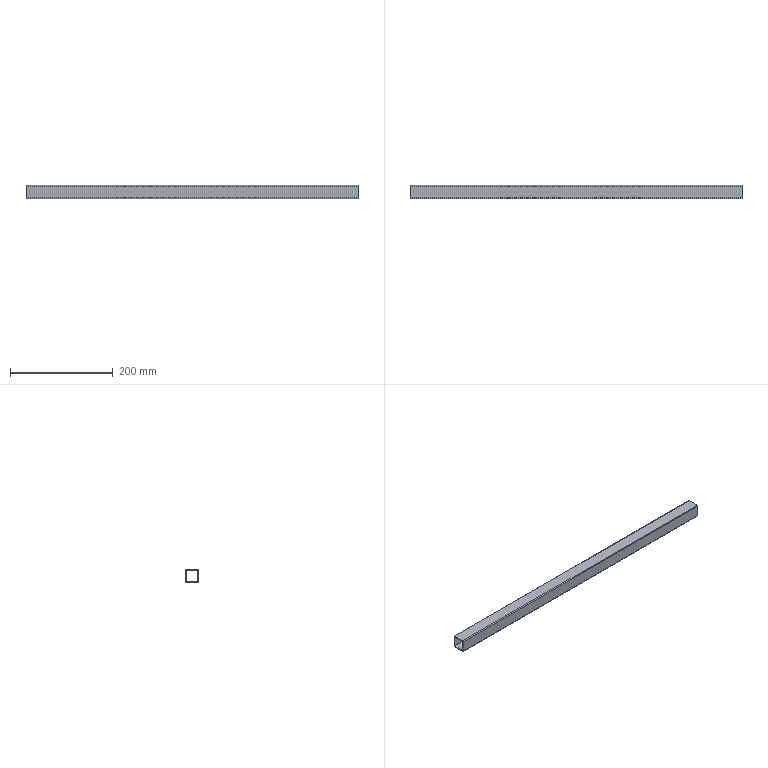Part | NX | features BREP 1 | 1 solid | 14 faces | box 647.7 x 25.4 x 25.4 mm | volume 113135 mm3 | plane 10 | cylinder 4 | commonest cylinder face diameters 3.175 x4
STEP:
#1=CARTESIAN_POINT('',(-323.85,12.7,-11.113));
#2=VERTEX_POINT('',#1);
#3=CARTESIAN_POINT('',(-323.85,12.7,11.113));
#4=VERTEX_POINT('',#3);
#5=CARTESIAN_POINT('',(-323.85,12.7,-11.113));
#6=DIRECTION('',(0.,0.,1.));
#7=VECTOR('',#6,1000.);
#8=LINE('',#5,#7);
#9=EDGE_CURVE('',#2,#4,#8,.T.);
#10=ORIENTED_EDGE('',*,*,#9,.F.);
#11=CARTESIAN_POINT('',(-323.85,11.113,-12.7));
#12=VERTEX_POINT('',#11);
#13=CARTESIAN_POINT('',(-323.85,11.113,-11.113));
#14=DIRECTION('',(-1.,0.,0.));
#15=DIRECTION('',(0.,1.,0.));
#16=AXIS2_PLACEMENT_3D('',#13,#14,#15);
#17=CIRCLE('',#16,1.587);
#18=EDGE_CURVE('',#2,#12,#17,.T.);
#19=ORIENTED_EDGE('',*,*,#18,.T.);
#20=CARTESIAN_POINT('',(-323.85,-11.113,-12.7));
#21=VERTEX_POINT('',#20);
#22=CARTESIAN_POINT('',(-323.85,-11.113,-12.7));
#23=DIRECTION('',(0.,1.,0.));
#24=VECTOR('',#23,1000.);
#25=LINE('',#22,#24);
#26=EDGE_CURVE('',#21,#12,#25,.T.);
#27=ORIENTED_EDGE('',*,*,#26,.F.);
#28=CARTESIAN_POINT('',(-323.85,-12.7,-11.113));
#29=VERTEX_POINT('',#28);
#30=CARTESIAN_POINT('',(-323.85,-11.113,-11.113));
#31=DIRECTION('',(-1.,0.,0.));
#32=DIRECTION('',(0.,0.,-1.));
#33=AXIS2_PLACEMENT_3D('',#30,#31,#32);
#34=CIRCLE('',#33,1.587);
#35=EDGE_CURVE('',#21,#29,#34,.T.);
#36=ORIENTED_EDGE('',*,*,#35,.T.);
#37=CARTESIAN_POINT('',(-323.85,-12.7,11.113));
#38=VERTEX_POINT('',#37);
#39=CARTESIAN_POINT('',(-323.85,-12.7,11.113));
#40=DIRECTION('',(0.,0.,-1.));
#41=VECTOR('',#40,1000.);
#42=LINE('',#39,#41);
#43=EDGE_CURVE('',#38,#29,#42,.T.);
#44=ORIENTED_EDGE('',*,*,#43,.F.);
#45=CARTESIAN_POINT('',(-323.85,-11.113,12.7));
#46=VERTEX_POINT('',#45);
#47=CARTESIAN_POINT('',(-323.85,-11.113,11.113));
#48=DIRECTION('',(-1.,0.,0.));
#49=DIRECTION('',(0.,-1.,0.));
#50=AXIS2_PLACEMENT_3D('',#47,#48,#49);
#51=CIRCLE('',#50,1.587);
#52=EDGE_CURVE('',#38,#46,#51,.T.);
#53=ORIENTED_EDGE('',*,*,#52,.T.);
#54=CARTESIAN_POINT('',(-323.85,11.113,12.7));
#55=VERTEX_POINT('',#54);
#56=CARTESIAN_POINT('',(-323.85,11.113,12.7));
#57=DIRECTION('',(0.,-1.,0.));
#58=VECTOR('',#57,1000.);
#59=LINE('',#56,#58);
#60=EDGE_CURVE('',#55,#46,#59,.T.);
#61=ORIENTED_EDGE('',*,*,#60,.F.);
#62=CARTESIAN_POINT('',(-323.85,11.113,11.113));
#63=DIRECTION('',(-1.,0.,0.));
#64=DIRECTION('',(0.,0.,1.));
#65=AXIS2_PLACEMENT_3D('',#62,#63,#64);
#66=CIRCLE('',#65,1.587);
#67=EDGE_CURVE('',#55,#4,#66,.T.);
#68=ORIENTED_EDGE('',*,*,#67,.T.);
#69=EDGE_LOOP('',(#10,#19,#27,#36,#44,#53,#61,#68));
#70=FACE_BOUND('',#69,.T.);
#71=CARTESIAN_POINT('',(-323.85,10.82,10.82));
#72=VERTEX_POINT('',#71);
#73=CARTESIAN_POINT('',(-323.85,10.82,-10.82));
#74=VERTEX_POINT('',#73);
#75=CARTESIAN_POINT('',(-323.85,10.82,10.82));
#76=DIRECTION('',(0.,0.,-1.));
#77=VECTOR('',#76,1000.);
#78=LINE('',#75,#77);
#79=EDGE_CURVE('',#72,#74,#78,.T.);
#80=ORIENTED_EDGE('',*,*,#79,.F.);
#81=CARTESIAN_POINT('',(-323.85,-10.82,10.82));
#82=VERTEX_POINT('',#81);
#83=CARTESIAN_POINT('',(-323.85,-10.82,10.82));
#84=DIRECTION('',(0.,1.,0.));
#85=VECTOR('',#84,1000.);
#86=LINE('',#83,#85);
#87=EDGE_CURVE('',#82,#72,#86,.T.);
#88=ORIENTED_EDGE('',*,*,#87,.F.);
#89=CARTESIAN_POINT('',(-323.85,-10.82,-10.82));
#90=VERTEX_POINT('',#89);
#91=CARTESIAN_POINT('',(-323.85,-10.82,-10.82));
#92=DIRECTION('',(0.,0.,1.));
#93=VECTOR('',#92,1000.);
#94=LINE('',#91,#93);
#95=EDGE_CURVE('',#90,#82,#94,.T.);
#96=ORIENTED_EDGE('',*,*,#95,.F.);
#97=CARTESIAN_POINT('',(-323.85,10.82,-10.82));
#98=DIRECTION('',(0.,-1.,0.));
#99=VECTOR('',#98,1000.);
#100=LINE('',#97,#99);
#101=EDGE_CURVE('',#74,#90,#100,.T.);
#102=ORIENTED_EDGE('',*,*,#101,.F.);
#103=EDGE_LOOP('',(#80,#88,#96,#102));
#104=FACE_BOUND('',#103,.T.);
#105=CARTESIAN_POINT('',(-323.85,0.,0.));
#106=DIRECTION('',(1.,0.,0.));
#107=DIRECTION('',(0.,1.,0.));
#108=AXIS2_PLACEMENT_3D('',#105,#106,#107);
#109=PLANE('',#108);
#110=ADVANCED_FACE('',(#70,#104),#109,.F.);
#111=CARTESIAN_POINT('',(323.85,-10.82,-10.82));
#112=VERTEX_POINT('',#111);
#113=CARTESIAN_POINT('',(-323.85,-10.82,-10.82));
#114=DIRECTION('',(1.,0.,0.));
#115=VECTOR('',#114,1000.);
#116=LINE('',#113,#115);
#117=EDGE_CURVE('',#90,#112,#116,.T.);
#118=ORIENTED_EDGE('',*,*,#117,.T.);
#119=CARTESIAN_POINT('',(323.85,10.82,-10.82));
#120=VERTEX_POINT('',#119);
#121=CARTESIAN_POINT('',(323.85,10.82,-10.82));
#122=DIRECTION('',(0.,-1.,0.));
#123=VECTOR('',#122,1000.);
#124=LINE('',#121,#123);
#125=EDGE_CURVE('',#120,#112,#124,.T.);
#126=ORIENTED_EDGE('',*,*,#125,.F.);
#127=CARTESIAN_POINT('',(-323.85,10.82,-10.82));
#128=DIRECTION('',(1.,0.,0.));
#129=VECTOR('',#128,1000.);
#130=LINE('',#127,#129);
#131=EDGE_CURVE('',#74,#120,#130,.T.);
#132=ORIENTED_EDGE('',*,*,#131,.F.);
#133=ORIENTED_EDGE('',*,*,#101,.T.);
#134=EDGE_LOOP('',(#118,#126,#132,#133));
#135=FACE_BOUND('',#134,.T.);
#136=CARTESIAN_POINT('',(-323.85,10.82,-10.82));
#137=DIRECTION('',(0.,0.,1.));
#138=DIRECTION('',(1.,0.,0.));
#139=AXIS2_PLACEMENT_3D('',#136,#137,#138);
#140=PLANE('',#139);
#141=ADVANCED_FACE('',(#135),#140,.T.);
#142=ORIENTED_EDGE('',*,*,#131,.T.);
#143=CARTESIAN_POINT('',(323.85,10.82,10.82));
#144=VERTEX_POINT('',#143);
#145=CARTESIAN_POINT('',(323.85,10.82,10.82));
#146=DIRECTION('',(0.,0.,-1.));
#147=VECTOR('',#146,1000.);
#148=LINE('',#145,#147);
#149=EDGE_CURVE('',#144,#120,#148,.T.);
#150=ORIENTED_EDGE('',*,*,#149,.F.);
#151=CARTESIAN_POINT('',(-323.85,10.82,10.82));
#152=DIRECTION('',(1.,0.,0.));
#153=VECTOR('',#152,1000.);
#154=LINE('',#151,#153);
#155=EDGE_CURVE('',#72,#144,#154,.T.);
#156=ORIENTED_EDGE('',*,*,#155,.F.);
#157=ORIENTED_EDGE('',*,*,#79,.T.);
#158=EDGE_LOOP('',(#142,#150,#156,#157));
#159=FACE_BOUND('',#158,.T.);
#160=CARTESIAN_POINT('',(-323.85,10.82,10.82));
#161=DIRECTION('',(0.,-1.,0.));
#162=DIRECTION('',(0.,0.,-1.));
#163=AXIS2_PLACEMENT_3D('',#160,#161,#162);
#164=PLANE('',#163);
#165=ADVANCED_FACE('',(#159),#164,.T.);
#166=ORIENTED_EDGE('',*,*,#155,.T.);
#167=CARTESIAN_POINT('',(323.85,-10.82,10.82));
#168=VERTEX_POINT('',#167);
#169=CARTESIAN_POINT('',(323.85,-10.82,10.82));
#170=DIRECTION('',(0.,1.,0.));
#171=VECTOR('',#170,1000.);
#172=LINE('',#169,#171);
#173=EDGE_CURVE('',#168,#144,#172,.T.);
#174=ORIENTED_EDGE('',*,*,#173,.F.);
#175=CARTESIAN_POINT('',(-323.85,-10.82,10.82));
#176=DIRECTION('',(1.,0.,0.));
#177=VECTOR('',#176,1000.);
#178=LINE('',#175,#177);
#179=EDGE_CURVE('',#82,#168,#178,.T.);
#180=ORIENTED_EDGE('',*,*,#179,.F.);
#181=ORIENTED_EDGE('',*,*,#87,.T.);
#182=EDGE_LOOP('',(#166,#174,#180,#181));
#183=FACE_BOUND('',#182,.T.);
#184=CARTESIAN_POINT('',(-323.85,-10.82,10.82));
#185=DIRECTION('',(0.,0.,-1.));
#186=DIRECTION('',(0.,-1.,0.));
#187=AXIS2_PLACEMENT_3D('',#184,#185,#186);
#188=PLANE('',#187);
#189=ADVANCED_FACE('',(#183),#188,.T.);
#190=ORIENTED_EDGE('',*,*,#179,.T.);
#191=CARTESIAN_POINT('',(323.85,-10.82,-10.82));
#192=DIRECTION('',(0.,0.,1.));
#193=VECTOR('',#192,1000.);
#194=LINE('',#191,#193);
#195=EDGE_CURVE('',#112,#168,#194,.T.);
#196=ORIENTED_EDGE('',*,*,#195,.F.);
#197=ORIENTED_EDGE('',*,*,#117,.F.);
#198=ORIENTED_EDGE('',*,*,#95,.T.);
#199=EDGE_LOOP('',(#190,#196,#197,#198));
#200=FACE_BOUND('',#199,.T.);
#201=CARTESIAN_POINT('',(-323.85,-10.82,-10.82));
#202=DIRECTION('',(0.,1.,0.));
#203=DIRECTION('',(1.,0.,0.));
#204=AXIS2_PLACEMENT_3D('',#201,#202,#203);
#205=PLANE('',#204);
#206=ADVANCED_FACE('',(#200),#205,.T.);
#207=CARTESIAN_POINT('',(323.85,11.113,12.7));
#208=VERTEX_POINT('',#207);
#209=CARTESIAN_POINT('',(323.85,-11.113,12.7));
#210=VERTEX_POINT('',#209);
#211=CARTESIAN_POINT('',(323.85,11.113,12.7));
#212=DIRECTION('',(0.,-1.,0.));
#213=VECTOR('',#212,1000.);
#214=LINE('',#211,#213);
#215=EDGE_CURVE('',#208,#210,#214,.T.);
#216=ORIENTED_EDGE('',*,*,#215,.T.);
#217=CARTESIAN_POINT('',(323.85,-12.7,11.113));
#218=VERTEX_POINT('',#217);
#219=CARTESIAN_POINT('',(323.85,-11.113,11.113));
#220=DIRECTION('',(1.,0.,0.));
#221=DIRECTION('',(0.,0.,1.));
#222=AXIS2_PLACEMENT_3D('',#219,#220,#221);
#223=CIRCLE('',#222,1.587);
#224=EDGE_CURVE('',#210,#218,#223,.T.);
#225=ORIENTED_EDGE('',*,*,#224,.T.);
#226=CARTESIAN_POINT('',(323.85,-12.7,-11.113));
#227=VERTEX_POINT('',#226);
#228=CARTESIAN_POINT('',(323.85,-12.7,11.113));
#229=DIRECTION('',(0.,0.,-1.));
#230=VECTOR('',#229,1000.);
#231=LINE('',#228,#230);
#232=EDGE_CURVE('',#218,#227,#231,.T.);
#233=ORIENTED_EDGE('',*,*,#232,.T.);
#234=CARTESIAN_POINT('',(323.85,-11.113,-12.7));
#235=VERTEX_POINT('',#234);
#236=CARTESIAN_POINT('',(323.85,-11.113,-11.113));
#237=DIRECTION('',(1.,0.,0.));
#238=DIRECTION('',(0.,-1.,0.));
#239=AXIS2_PLACEMENT_3D('',#236,#237,#238);
#240=CIRCLE('',#239,1.587);
#241=EDGE_CURVE('',#227,#235,#240,.T.);
#242=ORIENTED_EDGE('',*,*,#241,.T.);
#243=CARTESIAN_POINT('',(323.85,11.113,-12.7));
#244=VERTEX_POINT('',#243);
#245=CARTESIAN_POINT('',(323.85,-11.113,-12.7));
#246=DIRECTION('',(0.,1.,0.));
#247=VECTOR('',#246,1000.);
#248=LINE('',#245,#247);
#249=EDGE_CURVE('',#235,#244,#248,.T.);
#250=ORIENTED_EDGE('',*,*,#249,.T.);
#251=CARTESIAN_POINT('',(323.85,12.7,-11.113));
#252=VERTEX_POINT('',#251);
#253=CARTESIAN_POINT('',(323.85,11.113,-11.113));
#254=DIRECTION('',(1.,0.,0.));
#255=DIRECTION('',(0.,0.,-1.));
#256=AXIS2_PLACEMENT_3D('',#253,#254,#255);
#257=CIRCLE('',#256,1.587);
#258=EDGE_CURVE('',#244,#252,#257,.T.);
#259=ORIENTED_EDGE('',*,*,#258,.T.);
#260=CARTESIAN_POINT('',(323.85,12.7,11.113));
#261=VERTEX_POINT('',#260);
#262=CARTESIAN_POINT('',(323.85,12.7,-11.113));
#263=DIRECTION('',(0.,0.,1.));
#264=VECTOR('',#263,1000.);
#265=LINE('',#262,#264);
#266=EDGE_CURVE('',#252,#261,#265,.T.);
#267=ORIENTED_EDGE('',*,*,#266,.T.);
#268=CARTESIAN_POINT('',(323.85,11.113,11.113));
#269=DIRECTION('',(1.,0.,0.));
#270=DIRECTION('',(0.,1.,0.));
#271=AXIS2_PLACEMENT_3D('',#268,#269,#270);
#272=CIRCLE('',#271,1.587);
#273=EDGE_CURVE('',#261,#208,#272,.T.);
#274=ORIENTED_EDGE('',*,*,#273,.T.);
#275=EDGE_LOOP('',(#216,#225,#233,#242,#250,#259,#267,#274));
#276=FACE_BOUND('',#275,.T.);
#277=ORIENTED_EDGE('',*,*,#195,.T.);
#278=ORIENTED_EDGE('',*,*,#173,.T.);
#279=ORIENTED_EDGE('',*,*,#149,.T.);
#280=ORIENTED_EDGE('',*,*,#125,.T.);
#281=EDGE_LOOP('',(#277,#278,#279,#280));
#282=FACE_BOUND('',#281,.T.);
#283=CARTESIAN_POINT('',(323.85,0.,0.));
#284=DIRECTION('',(1.,0.,0.));
#285=DIRECTION('',(0.,1.,0.));
#286=AXIS2_PLACEMENT_3D('',#283,#284,#285);
#287=PLANE('',#286);
#288=ADVANCED_FACE('',(#276,#282),#287,.T.);
#289=ORIENTED_EDGE('',*,*,#273,.F.);
#290=CARTESIAN_POINT('',(323.85,12.7,11.113));
#291=DIRECTION('',(-1.,0.,0.));
#292=VECTOR('',#291,1000.);
#293=LINE('',#290,#292);
#294=EDGE_CURVE('',#261,#4,#293,.T.);
#295=ORIENTED_EDGE('',*,*,#294,.T.);
#296=ORIENTED_EDGE('',*,*,#67,.F.);
#297=CARTESIAN_POINT('',(323.85,11.113,12.7));
#298=DIRECTION('',(-1.,0.,0.));
#299=VECTOR('',#298,1000.);
#300=LINE('',#297,#299);
#301=EDGE_CURVE('',#208,#55,#300,.T.);
#302=ORIENTED_EDGE('',*,*,#301,.F.);
#303=EDGE_LOOP('',(#289,#295,#296,#302));
#304=FACE_BOUND('',#303,.T.);
#305=CARTESIAN_POINT('',(324.865,11.113,11.113));
#306=DIRECTION('',(-1.,0.,0.));
#307=DIRECTION('',(0.,0.,1.));
#308=AXIS2_PLACEMENT_3D('',#305,#306,#307);
#309=CYLINDRICAL_SURFACE('',#308,1.587);
#310=ADVANCED_FACE('',(#304),#309,.T.);
#311=ORIENTED_EDGE('',*,*,#60,.T.);
#312=CARTESIAN_POINT('',(323.85,-11.113,12.7));
#313=DIRECTION('',(-1.,0.,0.));
#314=VECTOR('',#313,1000.);
#315=LINE('',#312,#314);
#316=EDGE_CURVE('',#210,#46,#315,.T.);
#317=ORIENTED_EDGE('',*,*,#316,.F.);
#318=ORIENTED_EDGE('',*,*,#215,.F.);
#319=ORIENTED_EDGE('',*,*,#301,.T.);
#320=EDGE_LOOP('',(#311,#317,#318,#319));
#321=FACE_BOUND('',#320,.T.);
#322=CARTESIAN_POINT('',(-323.85,12.7,12.7));
#323=DIRECTION('',(0.,0.,1.));
#324=DIRECTION('',(1.,0.,0.));
#325=AXIS2_PLACEMENT_3D('',#322,#323,#324);
#326=PLANE('',#325);
#327=ADVANCED_FACE('',(#321),#326,.T.);
#328=ORIENTED_EDGE('',*,*,#224,.F.);
#329=ORIENTED_EDGE('',*,*,#316,.T.);
#330=ORIENTED_EDGE('',*,*,#52,.F.);
#331=CARTESIAN_POINT('',(323.85,-12.7,11.113));
#332=DIRECTION('',(-1.,0.,0.));
#333=VECTOR('',#332,1000.);
#334=LINE('',#331,#333);
#335=EDGE_CURVE('',#218,#38,#334,.T.);
#336=ORIENTED_EDGE('',*,*,#335,.F.);
#337=EDGE_LOOP('',(#328,#329,#330,#336));
#338=FACE_BOUND('',#337,.T.);
#339=CARTESIAN_POINT('',(324.865,-11.113,11.113));
#340=DIRECTION('',(-1.,0.,0.));
#341=DIRECTION('',(0.,-1.,0.));
#342=AXIS2_PLACEMENT_3D('',#339,#340,#341);
#343=CYLINDRICAL_SURFACE('',#342,1.587);
#344=ADVANCED_FACE('',(#338),#343,.T.);
#345=ORIENTED_EDGE('',*,*,#43,.T.);
#346=CARTESIAN_POINT('',(323.85,-12.7,-11.113));
#347=DIRECTION('',(-1.,0.,0.));
#348=VECTOR('',#347,1000.);
#349=LINE('',#346,#348);
#350=EDGE_CURVE('',#227,#29,#349,.T.);
#351=ORIENTED_EDGE('',*,*,#350,.F.);
#352=ORIENTED_EDGE('',*,*,#232,.F.);
#353=ORIENTED_EDGE('',*,*,#335,.T.);
#354=EDGE_LOOP('',(#345,#351,#352,#353));
#355=FACE_BOUND('',#354,.T.);
#356=CARTESIAN_POINT('',(-323.85,-12.7,12.7));
#357=DIRECTION('',(0.,-1.,0.));
#358=DIRECTION('',(0.,0.,-1.));
#359=AXIS2_PLACEMENT_3D('',#356,#357,#358);
#360=PLANE('',#359);
#361=ADVANCED_FACE('',(#355),#360,.T.);
#362=ORIENTED_EDGE('',*,*,#241,.F.);
#363=ORIENTED_EDGE('',*,*,#350,.T.);
#364=ORIENTED_EDGE('',*,*,#35,.F.);
#365=CARTESIAN_POINT('',(323.85,-11.113,-12.7));
#366=DIRECTION('',(-1.,0.,0.));
#367=VECTOR('',#366,1000.);
#368=LINE('',#365,#367);
#369=EDGE_CURVE('',#235,#21,#368,.T.);
#370=ORIENTED_EDGE('',*,*,#369,.F.);
#371=EDGE_LOOP('',(#362,#363,#364,#370));
#372=FACE_BOUND('',#371,.T.);
#373=CARTESIAN_POINT('',(324.865,-11.113,-11.113));
#374=DIRECTION('',(-1.,0.,0.));
#375=DIRECTION('',(0.,0.,-1.));
#376=AXIS2_PLACEMENT_3D('',#373,#374,#375);
#377=CYLINDRICAL_SURFACE('',#376,1.587);
#378=ADVANCED_FACE('',(#372),#377,.T.);
#379=ORIENTED_EDGE('',*,*,#249,.F.);
#380=ORIENTED_EDGE('',*,*,#369,.T.);
#381=ORIENTED_EDGE('',*,*,#26,.T.);
#382=CARTESIAN_POINT('',(323.85,11.113,-12.7));
#383=DIRECTION('',(-1.,0.,0.));
#384=VECTOR('',#383,1000.);
#385=LINE('',#382,#384);
#386=EDGE_CURVE('',#244,#12,#385,.T.);
#387=ORIENTED_EDGE('',*,*,#386,.F.);
#388=EDGE_LOOP('',(#379,#380,#381,#387));
#389=FACE_BOUND('',#388,.T.);
#390=CARTESIAN_POINT('',(-323.85,-12.7,-12.7));
#391=DIRECTION('',(0.,0.,-1.));
#392=DIRECTION('',(0.,-1.,0.));
#393=AXIS2_PLACEMENT_3D('',#390,#391,#392);
#394=PLANE('',#393);
#395=ADVANCED_FACE('',(#389),#394,.T.);
#396=ORIENTED_EDGE('',*,*,#258,.F.);
#397=ORIENTED_EDGE('',*,*,#386,.T.);
#398=ORIENTED_EDGE('',*,*,#18,.F.);
#399=CARTESIAN_POINT('',(323.85,12.7,-11.113));
#400=DIRECTION('',(-1.,0.,0.));
#401=VECTOR('',#400,1000.);
#402=LINE('',#399,#401);
#403=EDGE_CURVE('',#252,#2,#402,.T.);
#404=ORIENTED_EDGE('',*,*,#403,.F.);
#405=EDGE_LOOP('',(#396,#397,#398,#404));
#406=FACE_BOUND('',#405,.T.);
#407=CARTESIAN_POINT('',(324.865,11.113,-11.113));
#408=DIRECTION('',(-1.,0.,0.));
#409=DIRECTION('',(0.,1.,0.));
#410=AXIS2_PLACEMENT_3D('',#407,#408,#409);
#411=CYLINDRICAL_SURFACE('',#410,1.587);
#412=ADVANCED_FACE('',(#406),#411,.T.);
#413=ORIENTED_EDGE('',*,*,#266,.F.);
#414=ORIENTED_EDGE('',*,*,#403,.T.);
#415=ORIENTED_EDGE('',*,*,#9,.T.);
#416=ORIENTED_EDGE('',*,*,#294,.F.);
#417=EDGE_LOOP('',(#413,#414,#415,#416));
#418=FACE_BOUND('',#417,.T.);
#419=CARTESIAN_POINT('',(-323.85,12.7,-12.7));
#420=DIRECTION('',(0.,1.,0.));
#421=DIRECTION('',(1.,0.,0.));
#422=AXIS2_PLACEMENT_3D('',#419,#420,#421);
#423=PLANE('',#422);
#424=ADVANCED_FACE('',(#418),#423,.T.);
#425=CLOSED_SHELL('',(#110,#141,#165,#189,#206,#288,#310,#327,#344,#361,#378,#395,#412,#424));
#426=MANIFOLD_SOLID_BREP('',#425);
#427=(LENGTH_UNIT()NAMED_UNIT(*)SI_UNIT(.MILLI.,.METRE.));
#428=UNCERTAINTY_MEASURE_WITH_UNIT(LENGTH_MEASURE(0.00001),#427,'','');
#429=(NAMED_UNIT(*)PLANE_ANGLE_UNIT()SI_UNIT($,.RADIAN.));
#430=(NAMED_UNIT(*)SI_UNIT($,.STERADIAN.)SOLID_ANGLE_UNIT());
#431=(GEOMETRIC_REPRESENTATION_CONTEXT(3)GLOBAL_UNCERTAINTY_ASSIGNED_CONTEXT((#428))GLOBAL_UNIT_ASSIGNED_CONTEXT((#427,#429,#430))REPRESENTATION_CONTEXT('',''));
#432=ADVANCED_BREP_SHAPE_REPRESENTATION('',(#426),#431);